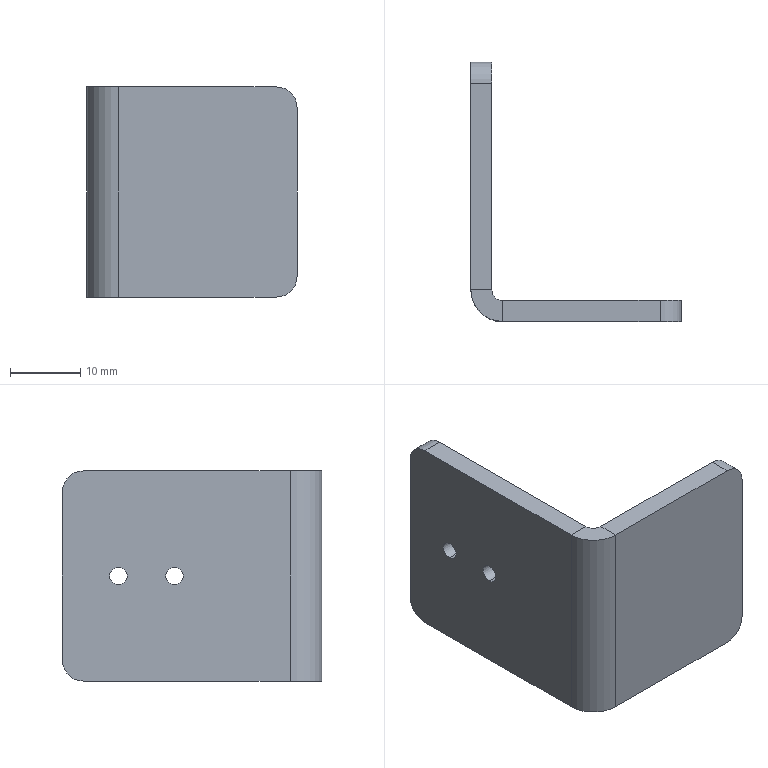Part | STEP file | 001-006-Pre-insertion mechanism drag chain mounting plate 2 | 1 solid | 22 faces | box 30 x 37 x 30 mm | volume 5591 mm3 | plane 12 | cylinder 10 | commonest cylinder face diameters 2.5 x4 6 x4 3 x1 9 x1